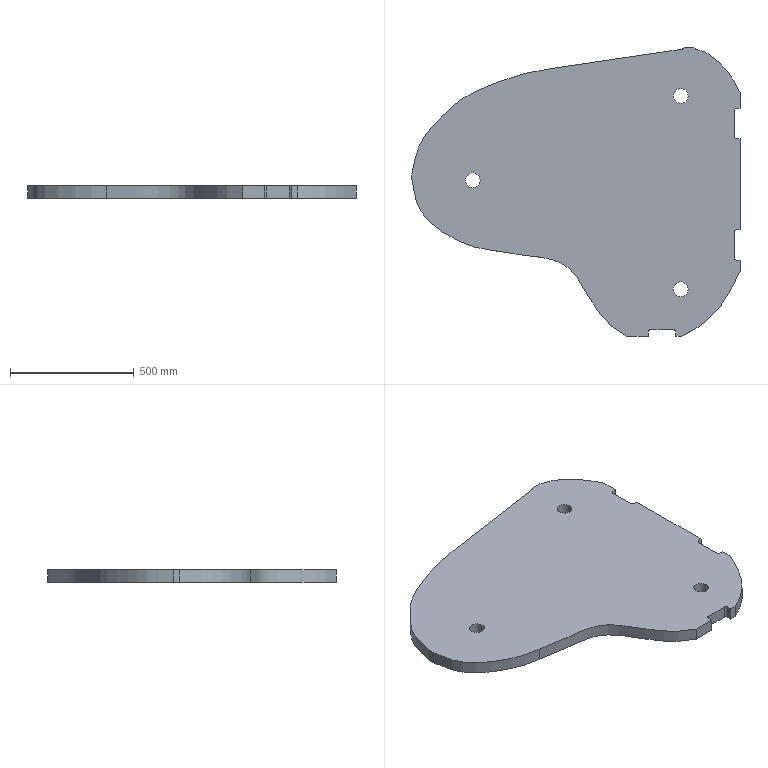Part | NX | features solid 2 | 1 solid | 34 faces | box 1325 x 1165 x 50 mm | volume 54786992 mm3 | plane 18 | cylinder 9 | spline 7 | commonest cylinder face diameters 20 x6 60 x3